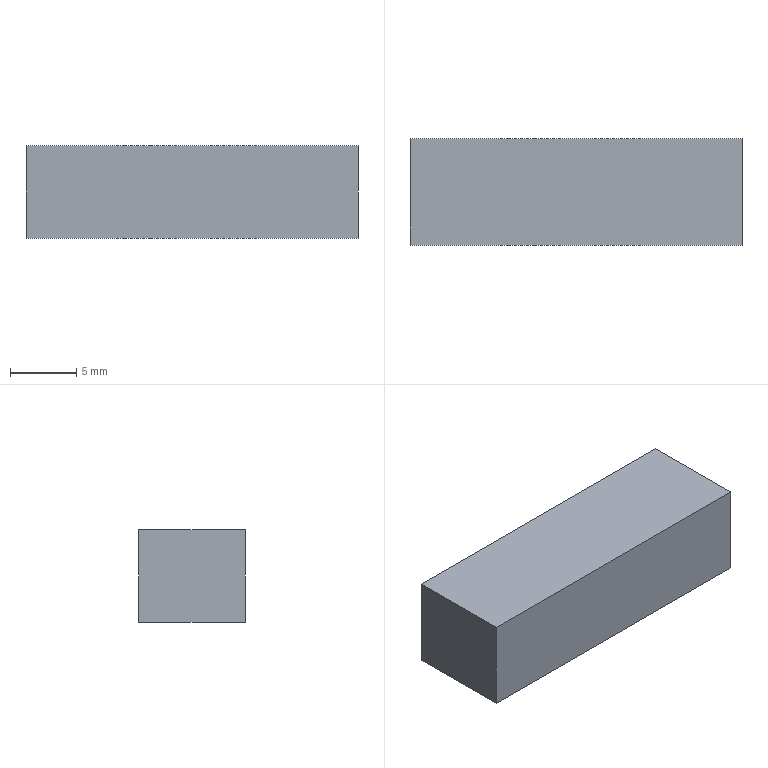Part | STEP file | Synchronous key | 1 solid | 6 faces | box 25 x 8 x 7 mm | volume 1400 mm3 | plane 6
STEP:
#1=CARTESIAN_POINT('',(-11.129,-7.627,7.));
#2=VERTEX_POINT('',#1);
#3=CARTESIAN_POINT('',(-11.129,0.3727,7.));
#4=VERTEX_POINT('',#3);
#5=CARTESIAN_POINT('',(-11.129,-7.627,7.));
#6=DIRECTION('',(0.,1.,0.));
#7=VECTOR('',#6,1000.);
#8=LINE('',#5,#7);
#9=EDGE_CURVE('',#2,#4,#8,.T.);
#10=ORIENTED_EDGE('',*,*,#9,.T.);
#11=CARTESIAN_POINT('',(-36.129,0.3727,7.));
#12=VERTEX_POINT('',#11);
#13=CARTESIAN_POINT('',(-36.129,0.3727,7.));
#14=DIRECTION('',(-1.,0.,0.));
#15=VECTOR('',#14,1000.);
#16=LINE('',#13,#15);
#17=EDGE_CURVE('',#4,#12,#16,.T.);
#18=ORIENTED_EDGE('',*,*,#17,.T.);
#19=CARTESIAN_POINT('',(-36.129,-7.627,7.));
#20=VERTEX_POINT('',#19);
#21=CARTESIAN_POINT('',(-36.129,-7.627,7.));
#22=DIRECTION('',(0.,-1.,0.));
#23=VECTOR('',#22,1000.);
#24=LINE('',#21,#23);
#25=EDGE_CURVE('',#12,#20,#24,.T.);
#26=ORIENTED_EDGE('',*,*,#25,.T.);
#27=CARTESIAN_POINT('',(-36.129,-7.627,7.));
#28=DIRECTION('',(1.,0.,0.));
#29=VECTOR('',#28,1000.);
#30=LINE('',#27,#29);
#31=EDGE_CURVE('',#20,#2,#30,.T.);
#32=ORIENTED_EDGE('',*,*,#31,.T.);
#33=EDGE_LOOP('',(#10,#18,#26,#32));
#34=FACE_OUTER_BOUND('',#33,.T.);
#35=CARTESIAN_POINT('',(-36.129,-7.627,7.));
#36=DIRECTION('',(0.,0.,1.));
#37=DIRECTION('',(1.,0.,0.));
#38=AXIS2_PLACEMENT_3D('',#35,#36,#37);
#39=PLANE('',#38);
#40=ADVANCED_FACE('',(#34),#39,.T.);
#41=CARTESIAN_POINT('',(-36.129,0.3727,0.));
#42=VERTEX_POINT('',#41);
#43=CARTESIAN_POINT('',(-36.129,0.3727,7.));
#44=DIRECTION('',(0.,0.,-1.));
#45=VECTOR('',#44,1000.);
#46=LINE('',#43,#45);
#47=EDGE_CURVE('',#12,#42,#46,.T.);
#48=ORIENTED_EDGE('',*,*,#47,.F.);
#49=ORIENTED_EDGE('',*,*,#17,.F.);
#50=CARTESIAN_POINT('',(-11.129,0.3727,0.));
#51=VERTEX_POINT('',#50);
#52=CARTESIAN_POINT('',(-11.129,0.3727,7.));
#53=DIRECTION('',(0.,0.,1.));
#54=VECTOR('',#53,1000.);
#55=LINE('',#52,#54);
#56=EDGE_CURVE('',#51,#4,#55,.T.);
#57=ORIENTED_EDGE('',*,*,#56,.F.);
#58=CARTESIAN_POINT('',(-36.129,0.3727,0.));
#59=DIRECTION('',(1.,0.,0.));
#60=VECTOR('',#59,1000.);
#61=LINE('',#58,#60);
#62=EDGE_CURVE('',#42,#51,#61,.T.);
#63=ORIENTED_EDGE('',*,*,#62,.F.);
#64=EDGE_LOOP('',(#48,#49,#57,#63));
#65=FACE_OUTER_BOUND('',#64,.T.);
#66=CARTESIAN_POINT('',(-36.129,0.3727,7.));
#67=DIRECTION('',(0.,-1.,0.));
#68=DIRECTION('',(0.,0.,-1.));
#69=AXIS2_PLACEMENT_3D('',#66,#67,#68);
#70=PLANE('',#69);
#71=ADVANCED_FACE('',(#65),#70,.F.);
#72=ORIENTED_EDGE('',*,*,#56,.T.);
#73=ORIENTED_EDGE('',*,*,#9,.F.);
#74=CARTESIAN_POINT('',(-11.129,-7.627,0.));
#75=VERTEX_POINT('',#74);
#76=CARTESIAN_POINT('',(-11.129,-7.627,7.));
#77=DIRECTION('',(0.,0.,1.));
#78=VECTOR('',#77,1000.);
#79=LINE('',#76,#78);
#80=EDGE_CURVE('',#75,#2,#79,.T.);
#81=ORIENTED_EDGE('',*,*,#80,.F.);
#82=CARTESIAN_POINT('',(-11.129,0.3727,0.));
#83=DIRECTION('',(0.,-1.,0.));
#84=VECTOR('',#83,1000.);
#85=LINE('',#82,#84);
#86=EDGE_CURVE('',#51,#75,#85,.T.);
#87=ORIENTED_EDGE('',*,*,#86,.F.);
#88=EDGE_LOOP('',(#72,#73,#81,#87));
#89=FACE_OUTER_BOUND('',#88,.T.);
#90=CARTESIAN_POINT('',(-11.129,0.3727,7.));
#91=DIRECTION('',(-1.,0.,0.));
#92=DIRECTION('',(0.,0.,1.));
#93=AXIS2_PLACEMENT_3D('',#90,#91,#92);
#94=PLANE('',#93);
#95=ADVANCED_FACE('',(#89),#94,.F.);
#96=ORIENTED_EDGE('',*,*,#80,.T.);
#97=ORIENTED_EDGE('',*,*,#31,.F.);
#98=CARTESIAN_POINT('',(-36.129,-7.627,0.));
#99=VERTEX_POINT('',#98);
#100=CARTESIAN_POINT('',(-36.129,-7.627,7.));
#101=DIRECTION('',(0.,0.,1.));
#102=VECTOR('',#101,1000.);
#103=LINE('',#100,#102);
#104=EDGE_CURVE('',#99,#20,#103,.T.);
#105=ORIENTED_EDGE('',*,*,#104,.F.);
#106=CARTESIAN_POINT('',(-36.129,-7.627,0.));
#107=DIRECTION('',(-1.,0.,0.));
#108=VECTOR('',#107,1000.);
#109=LINE('',#106,#108);
#110=EDGE_CURVE('',#75,#99,#109,.T.);
#111=ORIENTED_EDGE('',*,*,#110,.F.);
#112=EDGE_LOOP('',(#96,#97,#105,#111));
#113=FACE_OUTER_BOUND('',#112,.T.);
#114=CARTESIAN_POINT('',(-36.129,-7.627,7.));
#115=DIRECTION('',(0.,1.,0.));
#116=DIRECTION('',(0.,0.,1.));
#117=AXIS2_PLACEMENT_3D('',#114,#115,#116);
#118=PLANE('',#117);
#119=ADVANCED_FACE('',(#113),#118,.F.);
#120=ORIENTED_EDGE('',*,*,#104,.T.);
#121=ORIENTED_EDGE('',*,*,#25,.F.);
#122=ORIENTED_EDGE('',*,*,#47,.T.);
#123=CARTESIAN_POINT('',(-36.129,0.3727,0.));
#124=DIRECTION('',(0.,1.,0.));
#125=VECTOR('',#124,1000.);
#126=LINE('',#123,#125);
#127=EDGE_CURVE('',#99,#42,#126,.T.);
#128=ORIENTED_EDGE('',*,*,#127,.F.);
#129=EDGE_LOOP('',(#120,#121,#122,#128));
#130=FACE_OUTER_BOUND('',#129,.T.);
#131=CARTESIAN_POINT('',(-36.129,0.3727,7.));
#132=DIRECTION('',(1.,0.,0.));
#133=DIRECTION('',(0.,0.,-1.));
#134=AXIS2_PLACEMENT_3D('',#131,#132,#133);
#135=PLANE('',#134);
#136=ADVANCED_FACE('',(#130),#135,.F.);
#137=ORIENTED_EDGE('',*,*,#62,.T.);
#138=ORIENTED_EDGE('',*,*,#86,.T.);
#139=ORIENTED_EDGE('',*,*,#110,.T.);
#140=ORIENTED_EDGE('',*,*,#127,.T.);
#141=EDGE_LOOP('',(#137,#138,#139,#140));
#142=FACE_OUTER_BOUND('',#141,.T.);
#143=CARTESIAN_POINT('',(-36.129,-7.627,0.));
#144=DIRECTION('',(0.,0.,1.));
#145=DIRECTION('',(1.,0.,0.));
#146=AXIS2_PLACEMENT_3D('',#143,#144,#145);
#147=PLANE('',#146);
#148=ADVANCED_FACE('',(#142),#147,.F.);
#149=CLOSED_SHELL('',(#40,#71,#95,#119,#136,#148));
#150=MANIFOLD_SOLID_BREP('',#149);
#151=CARTESIAN_POINT('',(0.,0.,0.));
#152=DIRECTION('',(0.,0.,1.));
#153=DIRECTION('',(1.,0.,0.));
#154=AXIS2_PLACEMENT_3D('',#151,#152,#153);
#155=(LENGTH_UNIT()NAMED_UNIT(*)SI_UNIT(.MILLI.,.METRE.));
#156=UNCERTAINTY_MEASURE_WITH_UNIT(LENGTH_MEASURE(0.00001),#155,'','');
#157=(NAMED_UNIT(*)PLANE_ANGLE_UNIT()SI_UNIT($,.RADIAN.));
#158=(NAMED_UNIT(*)SI_UNIT($,.STERADIAN.)SOLID_ANGLE_UNIT());
#159=(GEOMETRIC_REPRESENTATION_CONTEXT(3)GLOBAL_UNCERTAINTY_ASSIGNED_CONTEXT((#156))GLOBAL_UNIT_ASSIGNED_CONTEXT((#155,#157,#158))REPRESENTATION_CONTEXT('',''));
#160=ADVANCED_BREP_SHAPE_REPRESENTATION('',(#150,#154),#159);